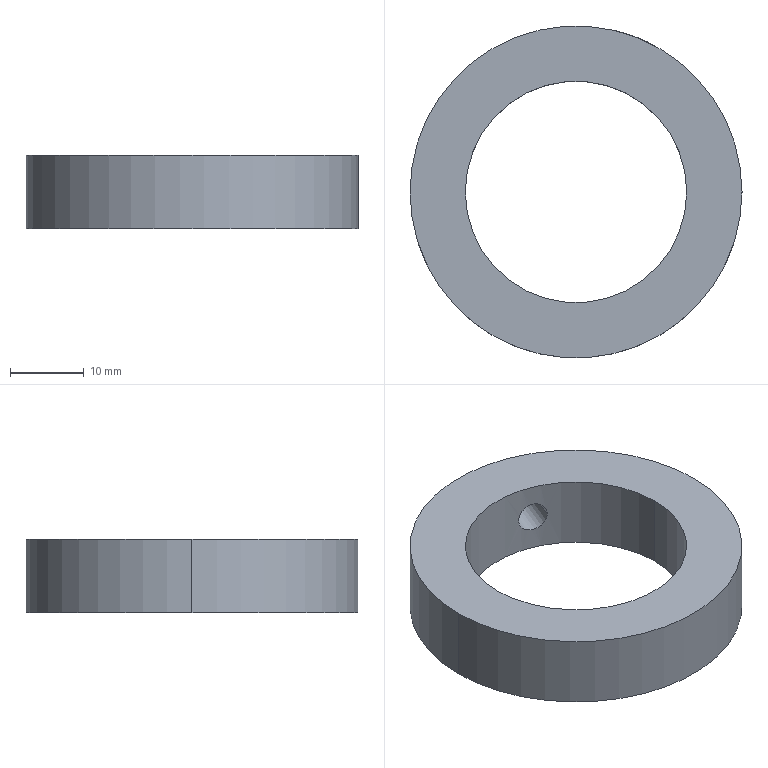Part | SolidWorks | features 3DProfileFeature 1, Extrusion 1, HoleWzd 1 | 1 solid | 8 faces | box 45 x 45 x 10 mm | volume 8732 mm3 | cylinder 6 | plane 2 | commonest cylinder face diameters 4.2 x2 30 x2 45 x2
STEP:
#1=CARTESIAN_POINT('',(3.587,14.565,5.069));
#2=VERTEX_POINT('',#1);
#3=CARTESIAN_POINT('',(7.484,13.,5.069));
#4=VERTEX_POINT('',#3);
#5=CARTESIAN_POINT('',(3.587,14.565,5.069));
#6=CARTESIAN_POINT('',(3.587,14.565,4.93));
#7=CARTESIAN_POINT('',(3.6,14.562,4.794));
#8=CARTESIAN_POINT('',(3.652,14.549,4.525));
#9=CARTESIAN_POINT('',(3.692,14.539,4.391));
#10=CARTESIAN_POINT('',(3.795,14.512,4.137));
#11=CARTESIAN_POINT('',(3.858,14.496,4.017));
#12=CARTESIAN_POINT('',(4.006,14.455,3.789));
#13=CARTESIAN_POINT('',(4.092,14.431,3.681));
#14=CARTESIAN_POINT('',(4.372,14.35,3.39));
#15=CARTESIAN_POINT('',(4.596,14.281,3.234));
#16=CARTESIAN_POINT('',(5.075,14.117,3.025));
#17=CARTESIAN_POINT('',(5.335,14.022,2.969));
#18=CARTESIAN_POINT('',(5.717,13.868,2.969));
#19=CARTESIAN_POINT('',(5.846,13.815,2.983));
#20=CARTESIAN_POINT('',(6.093,13.707,3.036));
#21=CARTESIAN_POINT('',(6.212,13.654,3.076));
#22=CARTESIAN_POINT('',(6.443,13.546,3.182));
#23=CARTESIAN_POINT('',(6.554,13.493,3.247));
#24=CARTESIAN_POINT('',(6.759,13.392,3.399));
#25=CARTESIAN_POINT('',(6.854,13.343,3.486));
#26=CARTESIAN_POINT('',(7.028,13.252,3.682));
#27=CARTESIAN_POINT('',(7.105,13.211,3.788));
#28=CARTESIAN_POINT('',(7.239,13.138,4.015));
#29=CARTESIAN_POINT('',(7.297,13.105,4.138));
#30=CARTESIAN_POINT('',(7.39,13.053,4.392));
#31=CARTESIAN_POINT('',(7.425,13.033,4.523));
#32=CARTESIAN_POINT('',(7.472,13.007,4.793));
#33=CARTESIAN_POINT('',(7.484,13.,4.932));
#34=CARTESIAN_POINT('',(7.484,13.,5.069));
#35=B_SPLINE_CURVE_WITH_KNOTS('',3,(#5,#6,#7,#8,#9,#10,#11,#12,#13,#14,#15,#16,#17,#18,#19,#20,#21,#22,#23,#24,#25,#26,#27,#28,#29,#30,#31,#32,#33,#34),.UNSPECIFIED.,.F.,.F.,(4,2,2,2,2,2,2,2,2,2,2,2,2,2,4),(0.,0.0004109,0.0008217,0.001233,0.001643,0.002465,0.003287,0.003698,0.004109,0.004519,0.00493,0.005341,0.005752,0.006163,0.006574),.UNSPECIFIED.);
#36=EDGE_CURVE('',#2,#4,#35,.T.);
#37=ORIENTED_EDGE('',*,*,#36,.T.);
#38=CARTESIAN_POINT('',(10.298,20.005,5.069));
#39=VERTEX_POINT('',#38);
#40=CARTESIAN_POINT('',(10.334,20.096,5.069));
#41=DIRECTION('',(0.3727,0.928,0.));
#42=VECTOR('',#41,1000.);
#43=LINE('',#40,#42);
#44=EDGE_CURVE('',#4,#39,#43,.T.);
#45=ORIENTED_EDGE('',*,*,#44,.T.);
#46=CARTESIAN_POINT('',(6.4,21.57,5.069));
#47=VERTEX_POINT('',#46);
#48=CARTESIAN_POINT('',(6.4,21.57,5.069));
#49=CARTESIAN_POINT('',(6.4,21.57,4.93));
#50=CARTESIAN_POINT('',(6.413,21.567,4.794));
#51=CARTESIAN_POINT('',(6.465,21.551,4.525));
#52=CARTESIAN_POINT('',(6.504,21.54,4.392));
#53=CARTESIAN_POINT('',(6.605,21.509,4.138));
#54=CARTESIAN_POINT('',(6.667,21.49,4.017));
#55=CARTESIAN_POINT('',(6.813,21.444,3.789));
#56=CARTESIAN_POINT('',(6.897,21.417,3.681));
#57=CARTESIAN_POINT('',(7.174,21.326,3.39));
#58=CARTESIAN_POINT('',(7.396,21.251,3.234));
#59=CARTESIAN_POINT('',(7.872,21.08,3.024));
#60=CARTESIAN_POINT('',(8.131,20.981,2.969));
#61=CARTESIAN_POINT('',(8.512,20.828,2.969));
#62=CARTESIAN_POINT('',(8.641,20.775,2.983));
#63=CARTESIAN_POINT('',(8.889,20.67,3.036));
#64=CARTESIAN_POINT('',(9.009,20.618,3.076));
#65=CARTESIAN_POINT('',(9.242,20.515,3.181));
#66=CARTESIAN_POINT('',(9.354,20.464,3.247));
#67=CARTESIAN_POINT('',(9.56,20.368,3.399));
#68=CARTESIAN_POINT('',(9.656,20.323,3.486));
#69=CARTESIAN_POINT('',(9.834,20.238,3.682));
#70=CARTESIAN_POINT('',(9.912,20.199,3.788));
#71=CARTESIAN_POINT('',(10.049,20.132,4.015));
#72=CARTESIAN_POINT('',(10.108,20.102,4.138));
#73=CARTESIAN_POINT('',(10.202,20.054,4.393));
#74=CARTESIAN_POINT('',(10.237,20.036,4.524));
#75=CARTESIAN_POINT('',(10.285,20.012,4.793));
#76=CARTESIAN_POINT('',(10.298,20.005,4.932));
#77=CARTESIAN_POINT('',(10.298,20.005,5.069));
#78=B_SPLINE_CURVE_WITH_KNOTS('',3,(#48,#49,#50,#51,#52,#53,#54,#55,#56,#57,#58,#59,#60,#61,#62,#63,#64,#65,#66,#67,#68,#69,#70,#71,#72,#73,#74,#75,#76,#77),.UNSPECIFIED.,.F.,.F.,(4,2,2,2,2,2,2,2,2,2,2,2,2,2,4),(0.,0.0004106,0.0008211,0.001232,0.001642,0.002463,0.003285,0.003695,0.004106,0.004516,0.004927,0.005337,0.005748,0.006159,0.006569),.UNSPECIFIED.);
#79=EDGE_CURVE('',#47,#39,#78,.T.);
#80=ORIENTED_EDGE('',*,*,#79,.F.);
#81=CARTESIAN_POINT('',(6.437,21.662,5.069));
#82=DIRECTION('',(0.3727,0.928,0.));
#83=VECTOR('',#82,1000.);
#84=LINE('',#81,#83);
#85=EDGE_CURVE('',#2,#47,#84,.T.);
#86=ORIENTED_EDGE('',*,*,#85,.F.);
#87=EDGE_LOOP('',(#37,#45,#80,#86));
#88=FACE_OUTER_BOUND('',#87,.T.);
#89=CARTESIAN_POINT('',(8.386,20.879,5.069));
#90=DIRECTION('',(0.3727,0.928,0.));
#91=DIRECTION('',(-0.928,0.3727,0.));
#92=AXIS2_PLACEMENT_3D('',#89,#90,#91);
#93=CYLINDRICAL_SURFACE('',#92,2.1);
#94=ADVANCED_FACE('',(#88),#93,.F.);
#95=CARTESIAN_POINT('',(-15.,0.,10.));
#96=VERTEX_POINT('',#95);
#97=CARTESIAN_POINT('',(15.,0.,10.));
#98=VERTEX_POINT('',#97);
#99=CARTESIAN_POINT('',(0.,0.,10.));
#100=DIRECTION('',(0.,0.,1.));
#101=DIRECTION('',(1.,0.,0.));
#102=AXIS2_PLACEMENT_3D('',#99,#100,#101);
#103=CIRCLE('',#102,15.);
#104=EDGE_CURVE('',#96,#98,#103,.T.);
#105=ORIENTED_EDGE('',*,*,#104,.T.);
#106=CARTESIAN_POINT('',(15.,0.,0.));
#107=VERTEX_POINT('',#106);
#108=CARTESIAN_POINT('',(15.,0.,10.));
#109=DIRECTION('',(0.,0.,-1.));
#110=VECTOR('',#109,1000.);
#111=LINE('',#108,#110);
#112=EDGE_CURVE('',#98,#107,#111,.T.);
#113=ORIENTED_EDGE('',*,*,#112,.T.);
#114=CARTESIAN_POINT('',(-15.,0.,0.));
#115=VERTEX_POINT('',#114);
#116=CARTESIAN_POINT('',(0.,0.,0.));
#117=DIRECTION('',(0.,0.,1.));
#118=DIRECTION('',(1.,0.,0.));
#119=AXIS2_PLACEMENT_3D('',#116,#117,#118);
#120=CIRCLE('',#119,15.);
#121=EDGE_CURVE('',#115,#107,#120,.T.);
#122=ORIENTED_EDGE('',*,*,#121,.F.);
#123=CARTESIAN_POINT('',(-15.,0.,10.));
#124=DIRECTION('',(0.,0.,-1.));
#125=VECTOR('',#124,1000.);
#126=LINE('',#123,#125);
#127=EDGE_CURVE('',#96,#115,#126,.T.);
#128=ORIENTED_EDGE('',*,*,#127,.F.);
#129=EDGE_LOOP('',(#105,#113,#122,#128));
#130=FACE_OUTER_BOUND('',#129,.T.);
#131=CARTESIAN_POINT('',(0.,0.,10.));
#132=DIRECTION('',(0.,0.,-1.));
#133=DIRECTION('',(-1.,0.,0.));
#134=AXIS2_PLACEMENT_3D('',#131,#132,#133);
#135=CYLINDRICAL_SURFACE('',#134,15.);
#136=ADVANCED_FACE('',(#130),#135,.F.);
#137=ORIENTED_EDGE('',*,*,#79,.T.);
#138=CARTESIAN_POINT('',(10.298,20.005,5.069));
#139=CARTESIAN_POINT('',(10.298,20.005,5.343));
#140=CARTESIAN_POINT('',(10.249,20.031,5.62));
#141=CARTESIAN_POINT('',(10.061,20.125,6.125));
#142=CARTESIAN_POINT('',(9.921,20.196,6.359));
#143=CARTESIAN_POINT('',(9.659,20.322,6.65));
#144=CARTESIAN_POINT('',(9.561,20.368,6.739));
#145=CARTESIAN_POINT('',(9.354,20.464,6.891));
#146=CARTESIAN_POINT('',(9.244,20.514,6.956));
#147=CARTESIAN_POINT('',(9.012,20.617,7.061));
#148=CARTESIAN_POINT('',(8.889,20.67,7.102));
#149=CARTESIAN_POINT('',(8.642,20.775,7.155));
#150=CARTESIAN_POINT('',(8.516,20.827,7.169));
#151=CARTESIAN_POINT('',(8.258,20.93,7.169));
#152=CARTESIAN_POINT('',(8.131,20.98,7.156));
#153=CARTESIAN_POINT('',(7.88,21.075,7.103));
#154=CARTESIAN_POINT('',(7.755,21.122,7.062));
#155=CARTESIAN_POINT('',(7.516,21.208,6.957));
#156=CARTESIAN_POINT('',(7.402,21.248,6.893));
#157=CARTESIAN_POINT('',(7.185,21.322,6.74));
#158=CARTESIAN_POINT('',(7.083,21.356,6.652));
#159=CARTESIAN_POINT('',(6.806,21.447,6.362));
#160=CARTESIAN_POINT('',(6.656,21.493,6.128));
#161=CARTESIAN_POINT('',(6.454,21.555,5.623));
#162=CARTESIAN_POINT('',(6.4,21.57,5.347));
#163=CARTESIAN_POINT('',(6.4,21.57,5.069));
#164=B_SPLINE_CURVE_WITH_KNOTS('',3,(#138,#139,#140,#141,#142,#143,#144,#145,#146,#147,#148,#149,#150,#151,#152,#153,#154,#155,#156,#157,#158,#159,#160,#161,#162,#163),.UNSPECIFIED.,.F.,.F.,(4,2,2,2,2,2,2,2,2,2,2,2,4),(0.006569,0.00739,0.008211,0.008622,0.009032,0.009442,0.009853,0.01026,0.01067,0.01108,0.01149,0.01232,0.01314),.UNSPECIFIED.);
#165=EDGE_CURVE('',#39,#47,#164,.T.);
#166=ORIENTED_EDGE('',*,*,#165,.T.);
#167=EDGE_LOOP('',(#137,#166));
#168=FACE_BOUND('',#167,.T.);
#169=CARTESIAN_POINT('',(22.5,0.,10.));
#170=VERTEX_POINT('',#169);
#171=CARTESIAN_POINT('',(-22.5,0.,10.));
#172=VERTEX_POINT('',#171);
#173=CARTESIAN_POINT('',(0.,0.,10.));
#174=DIRECTION('',(0.,0.,1.));
#175=DIRECTION('',(1.,0.,0.));
#176=AXIS2_PLACEMENT_3D('',#173,#174,#175);
#177=CIRCLE('',#176,22.5);
#178=EDGE_CURVE('',#170,#172,#177,.T.);
#179=ORIENTED_EDGE('',*,*,#178,.F.);
#180=CARTESIAN_POINT('',(22.5,0.,0.));
#181=VERTEX_POINT('',#180);
#182=CARTESIAN_POINT('',(22.5,0.,10.));
#183=DIRECTION('',(0.,0.,-1.));
#184=VECTOR('',#183,1000.);
#185=LINE('',#182,#184);
#186=EDGE_CURVE('',#170,#181,#185,.T.);
#187=ORIENTED_EDGE('',*,*,#186,.T.);
#188=CARTESIAN_POINT('',(-22.5,0.,0.));
#189=VERTEX_POINT('',#188);
#190=CARTESIAN_POINT('',(0.,0.,0.));
#191=DIRECTION('',(0.,0.,1.));
#192=DIRECTION('',(1.,0.,0.));
#193=AXIS2_PLACEMENT_3D('',#190,#191,#192);
#194=CIRCLE('',#193,22.5);
#195=EDGE_CURVE('',#181,#189,#194,.T.);
#196=ORIENTED_EDGE('',*,*,#195,.T.);
#197=CARTESIAN_POINT('',(-22.5,0.,10.));
#198=DIRECTION('',(0.,0.,-1.));
#199=VECTOR('',#198,1000.);
#200=LINE('',#197,#199);
#201=EDGE_CURVE('',#172,#189,#200,.T.);
#202=ORIENTED_EDGE('',*,*,#201,.F.);
#203=EDGE_LOOP('',(#179,#187,#196,#202));
#204=FACE_OUTER_BOUND('',#203,.T.);
#205=CARTESIAN_POINT('',(0.,0.,10.));
#206=DIRECTION('',(0.,0.,-1.));
#207=DIRECTION('',(-1.,0.,0.));
#208=AXIS2_PLACEMENT_3D('',#205,#206,#207);
#209=CYLINDRICAL_SURFACE('',#208,22.5);
#210=ADVANCED_FACE('',(#168,#204),#209,.T.);
#211=CARTESIAN_POINT('',(0.,0.,10.));
#212=DIRECTION('',(0.,0.,1.));
#213=DIRECTION('',(1.,0.,0.));
#214=AXIS2_PLACEMENT_3D('',#211,#212,#213);
#215=CIRCLE('',#214,22.5);
#216=EDGE_CURVE('',#172,#170,#215,.T.);
#217=ORIENTED_EDGE('',*,*,#216,.T.);
#218=ORIENTED_EDGE('',*,*,#178,.T.);
#219=EDGE_LOOP('',(#217,#218));
#220=FACE_OUTER_BOUND('',#219,.T.);
#221=ORIENTED_EDGE('',*,*,#104,.F.);
#222=CARTESIAN_POINT('',(0.,0.,10.));
#223=DIRECTION('',(0.,0.,1.));
#224=DIRECTION('',(1.,0.,0.));
#225=AXIS2_PLACEMENT_3D('',#222,#223,#224);
#226=CIRCLE('',#225,15.);
#227=EDGE_CURVE('',#98,#96,#226,.T.);
#228=ORIENTED_EDGE('',*,*,#227,.F.);
#229=EDGE_LOOP('',(#221,#228));
#230=FACE_BOUND('',#229,.T.);
#231=CARTESIAN_POINT('',(0.,0.,10.));
#232=DIRECTION('',(0.,0.,1.));
#233=DIRECTION('',(1.,0.,0.));
#234=AXIS2_PLACEMENT_3D('',#231,#232,#233);
#235=PLANE('',#234);
#236=ADVANCED_FACE('',(#220,#230),#235,.T.);
#237=CARTESIAN_POINT('',(0.,0.,0.));
#238=DIRECTION('',(0.,0.,1.));
#239=DIRECTION('',(1.,0.,0.));
#240=AXIS2_PLACEMENT_3D('',#237,#238,#239);
#241=CIRCLE('',#240,22.5);
#242=EDGE_CURVE('',#189,#181,#241,.T.);
#243=ORIENTED_EDGE('',*,*,#242,.F.);
#244=ORIENTED_EDGE('',*,*,#195,.F.);
#245=EDGE_LOOP('',(#243,#244));
#246=FACE_OUTER_BOUND('',#245,.T.);
#247=ORIENTED_EDGE('',*,*,#121,.T.);
#248=CARTESIAN_POINT('',(0.,0.,0.));
#249=DIRECTION('',(0.,0.,1.));
#250=DIRECTION('',(1.,0.,0.));
#251=AXIS2_PLACEMENT_3D('',#248,#249,#250);
#252=CIRCLE('',#251,15.);
#253=EDGE_CURVE('',#107,#115,#252,.T.);
#254=ORIENTED_EDGE('',*,*,#253,.T.);
#255=EDGE_LOOP('',(#247,#254));
#256=FACE_BOUND('',#255,.T.);
#257=CARTESIAN_POINT('',(0.,0.,0.));
#258=DIRECTION('',(0.,0.,1.));
#259=DIRECTION('',(1.,0.,0.));
#260=AXIS2_PLACEMENT_3D('',#257,#258,#259);
#261=PLANE('',#260);
#262=ADVANCED_FACE('',(#246,#256),#261,.F.);
#263=ORIENTED_EDGE('',*,*,#186,.F.);
#264=ORIENTED_EDGE('',*,*,#216,.F.);
#265=ORIENTED_EDGE('',*,*,#201,.T.);
#266=ORIENTED_EDGE('',*,*,#242,.T.);
#267=EDGE_LOOP('',(#263,#264,#265,#266));
#268=FACE_OUTER_BOUND('',#267,.T.);
#269=CARTESIAN_POINT('',(0.,0.,10.));
#270=DIRECTION('',(0.,0.,-1.));
#271=DIRECTION('',(-1.,0.,0.));
#272=AXIS2_PLACEMENT_3D('',#269,#270,#271);
#273=CYLINDRICAL_SURFACE('',#272,22.5);
#274=ADVANCED_FACE('',(#268),#273,.T.);
#275=ORIENTED_EDGE('',*,*,#112,.F.);
#276=ORIENTED_EDGE('',*,*,#227,.T.);
#277=ORIENTED_EDGE('',*,*,#127,.T.);
#278=ORIENTED_EDGE('',*,*,#253,.F.);
#279=EDGE_LOOP('',(#275,#276,#277,#278));
#280=FACE_OUTER_BOUND('',#279,.T.);
#281=ORIENTED_EDGE('',*,*,#36,.F.);
#282=CARTESIAN_POINT('',(7.484,13.,5.069));
#283=CARTESIAN_POINT('',(7.484,13.,5.343));
#284=CARTESIAN_POINT('',(7.436,13.028,5.62));
#285=CARTESIAN_POINT('',(7.298,13.105,5.999));
#286=CARTESIAN_POINT('',(7.24,13.137,6.121));
#287=CARTESIAN_POINT('',(7.105,13.211,6.351));
#288=CARTESIAN_POINT('',(7.028,13.252,6.456));
#289=CARTESIAN_POINT('',(6.856,13.342,6.65));
#290=CARTESIAN_POINT('',(6.759,13.391,6.739));
#291=CARTESIAN_POINT('',(6.554,13.493,6.891));
#292=CARTESIAN_POINT('',(6.446,13.545,6.956));
#293=CARTESIAN_POINT('',(6.215,13.653,7.061));
#294=CARTESIAN_POINT('',(6.093,13.707,7.102));
#295=CARTESIAN_POINT('',(5.847,13.814,7.155));
#296=CARTESIAN_POINT('',(5.721,13.867,7.169));
#297=CARTESIAN_POINT('',(5.463,13.971,7.169));
#298=CARTESIAN_POINT('',(5.336,14.02,7.156));
#299=CARTESIAN_POINT('',(5.083,14.113,7.102));
#300=CARTESIAN_POINT('',(4.957,14.158,7.062));
#301=CARTESIAN_POINT('',(4.717,14.24,6.957));
#302=CARTESIAN_POINT('',(4.602,14.277,6.892));
#303=CARTESIAN_POINT('',(4.383,14.346,6.74));
#304=CARTESIAN_POINT('',(4.279,14.377,6.652));
#305=CARTESIAN_POINT('',(3.999,14.458,6.362));
#306=CARTESIAN_POINT('',(3.847,14.499,6.128));
#307=CARTESIAN_POINT('',(3.642,14.552,5.623));
#308=CARTESIAN_POINT('',(3.587,14.565,5.347));
#309=CARTESIAN_POINT('',(3.587,14.565,5.069));
#310=B_SPLINE_CURVE_WITH_KNOTS('',3,(#282,#283,#284,#285,#286,#287,#288,#289,#290,#291,#292,#293,#294,#295,#296,#297,#298,#299,#300,#301,#302,#303,#304,#305,#306,#307,#308,#309),.UNSPECIFIED.,.F.,.F.,(4,2,2,2,2,2,2,2,2,2,2,2,2,4),(0.006574,0.007395,0.007806,0.008217,0.008627,0.009038,0.009449,0.00986,0.01027,0.01068,0.01109,0.0115,0.01232,0.01315),.UNSPECIFIED.);
#311=EDGE_CURVE('',#4,#2,#310,.T.);
#312=ORIENTED_EDGE('',*,*,#311,.F.);
#313=EDGE_LOOP('',(#281,#312));
#314=FACE_BOUND('',#313,.T.);
#315=CARTESIAN_POINT('',(0.,0.,10.));
#316=DIRECTION('',(0.,0.,-1.));
#317=DIRECTION('',(-1.,0.,0.));
#318=AXIS2_PLACEMENT_3D('',#315,#316,#317);
#319=CYLINDRICAL_SURFACE('',#318,15.);
#320=ADVANCED_FACE('',(#280,#314),#319,.F.);
#321=ORIENTED_EDGE('',*,*,#44,.F.);
#322=ORIENTED_EDGE('',*,*,#311,.T.);
#323=ORIENTED_EDGE('',*,*,#85,.T.);
#324=ORIENTED_EDGE('',*,*,#165,.F.);
#325=EDGE_LOOP('',(#321,#322,#323,#324));
#326=FACE_OUTER_BOUND('',#325,.T.);
#327=CARTESIAN_POINT('',(8.386,20.879,5.069));
#328=DIRECTION('',(0.3727,0.928,0.));
#329=DIRECTION('',(-0.928,0.3727,0.));
#330=AXIS2_PLACEMENT_3D('',#327,#328,#329);
#331=CYLINDRICAL_SURFACE('',#330,2.1);
#332=ADVANCED_FACE('',(#326),#331,.F.);
#333=CLOSED_SHELL('',(#94,#136,#210,#236,#262,#274,#320,#332));
#334=MANIFOLD_SOLID_BREP('',#333);
#335=CARTESIAN_POINT('',(0.,0.,0.));
#336=DIRECTION('',(0.,0.,1.));
#337=DIRECTION('',(1.,0.,0.));
#338=AXIS2_PLACEMENT_3D('',#335,#336,#337);
#339=(LENGTH_UNIT()NAMED_UNIT(*)SI_UNIT(.MILLI.,.METRE.));
#340=UNCERTAINTY_MEASURE_WITH_UNIT(LENGTH_MEASURE(0.00001),#339,'','');
#341=(NAMED_UNIT(*)PLANE_ANGLE_UNIT()SI_UNIT($,.RADIAN.));
#342=(NAMED_UNIT(*)SI_UNIT($,.STERADIAN.)SOLID_ANGLE_UNIT());
#343=(GEOMETRIC_REPRESENTATION_CONTEXT(3)GLOBAL_UNCERTAINTY_ASSIGNED_CONTEXT((#340))GLOBAL_UNIT_ASSIGNED_CONTEXT((#339,#341,#342))REPRESENTATION_CONTEXT('',''));
#344=ADVANCED_BREP_SHAPE_REPRESENTATION('',(#334,#338),#343);